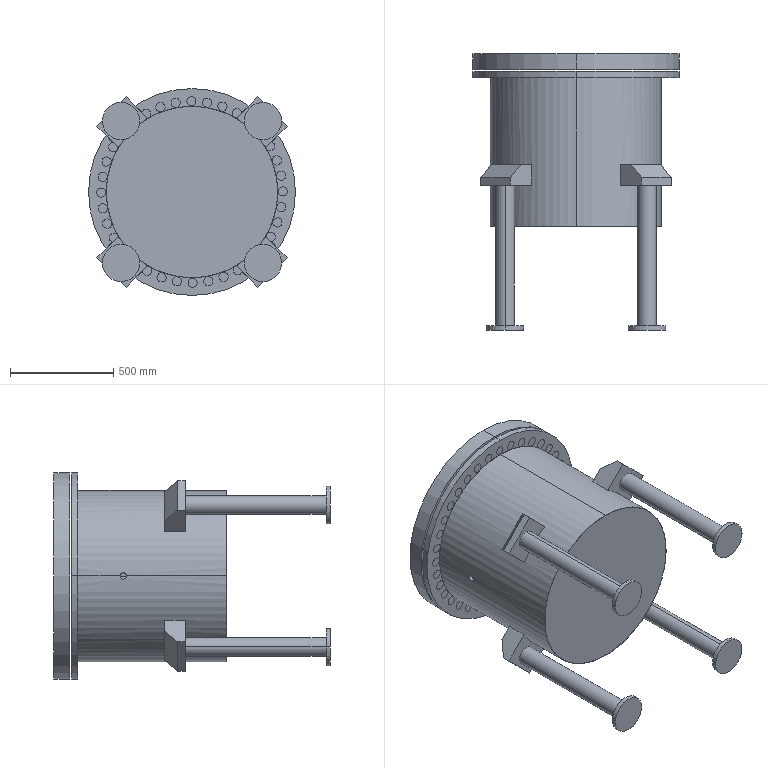Part | SolidWorks | features ICE 9, CirPattern 2, Extrusion 1, Shell 1 | 5 solids | 238 faces | box 1000 x 1336 x 1000 mm | volume 288874329 mm3 | cylinder 156 | plane 82 | commonest cylinder face diameters 44.371 x90 90 x16 180.752 x16 1000 x10 30 x8 800 x8